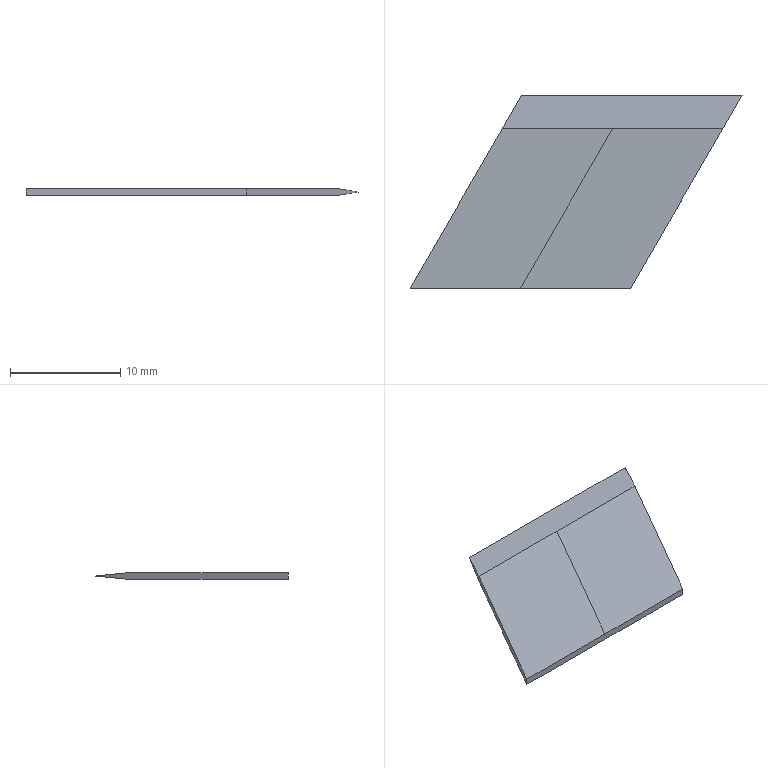Part | SolidWorks | features PLine 2, Extrusion 1, ICE 1, MirrorPattern 1 | 1 solid | 9 faces | box 30.104 x 17.5 x 0.6 mm | volume 192 mm3 | plane 9
STEP:
#1=CARTESIAN_POINT('',(10.,0.,0.6));
#2=VERTEX_POINT('',#1);
#3=CARTESIAN_POINT('',(18.372,14.5,0.6));
#4=VERTEX_POINT('',#3);
#5=CARTESIAN_POINT('',(7.5,-4.33,0.6));
#6=DIRECTION('',(0.5,0.866,0.));
#7=VECTOR('',#6,1000.);
#8=LINE('',#5,#7);
#9=EDGE_CURVE('',#2,#4,#8,.T.);
#10=ORIENTED_EDGE('',*,*,#9,.F.);
#11=CARTESIAN_POINT('',(20.,0.,0.6));
#12=VERTEX_POINT('',#11);
#13=CARTESIAN_POINT('',(20.,0.,0.6));
#14=DIRECTION('',(1.,0.,0.));
#15=VECTOR('',#14,1000.);
#16=LINE('',#13,#15);
#17=EDGE_CURVE('',#2,#12,#16,.T.);
#18=ORIENTED_EDGE('',*,*,#17,.T.);
#19=CARTESIAN_POINT('',(28.372,14.5,0.6));
#20=VERTEX_POINT('',#19);
#21=CARTESIAN_POINT('',(30.104,17.5,0.6));
#22=DIRECTION('',(0.5,0.866,0.));
#23=VECTOR('',#22,1000.);
#24=LINE('',#21,#23);
#25=EDGE_CURVE('',#12,#20,#24,.T.);
#26=ORIENTED_EDGE('',*,*,#25,.T.);
#27=CARTESIAN_POINT('',(30.104,14.5,0.6));
#28=DIRECTION('',(-1.,0.,0.));
#29=VECTOR('',#28,1000.);
#30=LINE('',#27,#29);
#31=EDGE_CURVE('',#20,#4,#30,.T.);
#32=ORIENTED_EDGE('',*,*,#31,.T.);
#33=EDGE_LOOP('',(#10,#18,#26,#32));
#34=FACE_OUTER_BOUND('',#33,.T.);
#35=CARTESIAN_POINT('',(0.,0.,0.6));
#36=DIRECTION('',(0.,0.,-1.));
#37=DIRECTION('',(-1.,0.,0.));
#38=AXIS2_PLACEMENT_3D('',#35,#36,#37);
#39=PLANE('',#38);
#40=ADVANCED_FACE('',(#34),#39,.F.);
#41=CARTESIAN_POINT('',(10.,0.,0.));
#42=VERTEX_POINT('',#41);
#43=CARTESIAN_POINT('',(20.,0.,0.));
#44=VERTEX_POINT('',#43);
#45=CARTESIAN_POINT('',(20.,0.,0.));
#46=DIRECTION('',(1.,0.,0.));
#47=VECTOR('',#46,1000.);
#48=LINE('',#45,#47);
#49=EDGE_CURVE('',#42,#44,#48,.T.);
#50=ORIENTED_EDGE('',*,*,#49,.F.);
#51=CARTESIAN_POINT('',(18.372,14.5,0.));
#52=VERTEX_POINT('',#51);
#53=CARTESIAN_POINT('',(7.5,-4.33,0.));
#54=DIRECTION('',(0.5,0.866,0.));
#55=VECTOR('',#54,1000.);
#56=LINE('',#53,#55);
#57=EDGE_CURVE('',#42,#52,#56,.T.);
#58=ORIENTED_EDGE('',*,*,#57,.T.);
#59=CARTESIAN_POINT('',(28.372,14.5,0.));
#60=VERTEX_POINT('',#59);
#61=CARTESIAN_POINT('',(0.,14.5,0.));
#62=DIRECTION('',(1.,0.,0.));
#63=VECTOR('',#62,1000.);
#64=LINE('',#61,#63);
#65=EDGE_CURVE('',#52,#60,#64,.T.);
#66=ORIENTED_EDGE('',*,*,#65,.T.);
#67=CARTESIAN_POINT('',(30.104,17.5,0.));
#68=DIRECTION('',(0.5,0.866,0.));
#69=VECTOR('',#68,1000.);
#70=LINE('',#67,#69);
#71=EDGE_CURVE('',#44,#60,#70,.T.);
#72=ORIENTED_EDGE('',*,*,#71,.F.);
#73=EDGE_LOOP('',(#50,#58,#66,#72));
#74=FACE_OUTER_BOUND('',#73,.T.);
#75=CARTESIAN_POINT('',(0.,0.,0.));
#76=DIRECTION('',(0.,0.,-1.));
#77=DIRECTION('',(-1.,0.,0.));
#78=AXIS2_PLACEMENT_3D('',#75,#76,#77);
#79=PLANE('',#78);
#80=ADVANCED_FACE('',(#74),#79,.T.);
#81=CARTESIAN_POINT('',(30.104,17.5,0.3));
#82=VERTEX_POINT('',#81);
#83=CARTESIAN_POINT('',(30.117,17.522,0.3022));
#84=DIRECTION('',(-0.4981,-0.8628,-0.08628));
#85=VECTOR('',#84,1000.);
#86=LINE('',#83,#85);
#87=EDGE_CURVE('',#82,#60,#86,.T.);
#88=ORIENTED_EDGE('',*,*,#87,.F.);
#89=CARTESIAN_POINT('',(30.091,17.478,0.3022));
#90=DIRECTION('',(-0.4981,-0.8628,0.08628));
#91=VECTOR('',#90,1000.);
#92=LINE('',#89,#91);
#93=EDGE_CURVE('',#82,#20,#92,.T.);
#94=ORIENTED_EDGE('',*,*,#93,.T.);
#95=ORIENTED_EDGE('',*,*,#25,.F.);
#96=CARTESIAN_POINT('',(20.,0.,0.6));
#97=DIRECTION('',(0.,0.,-1.));
#98=VECTOR('',#97,1000.);
#99=LINE('',#96,#98);
#100=EDGE_CURVE('',#12,#44,#99,.T.);
#101=ORIENTED_EDGE('',*,*,#100,.T.);
#102=ORIENTED_EDGE('',*,*,#71,.T.);
#103=EDGE_LOOP('',(#88,#94,#95,#101,#102));
#104=FACE_OUTER_BOUND('',#103,.T.);
#105=CARTESIAN_POINT('',(30.104,17.5,0.6));
#106=DIRECTION('',(-0.866,0.5,0.));
#107=DIRECTION('',(-0.5,-0.866,0.));
#108=AXIS2_PLACEMENT_3D('',#105,#106,#107);
#109=PLANE('',#108);
#110=ADVANCED_FACE('',(#104),#109,.F.);
#111=CARTESIAN_POINT('',(8.372,14.5,0.6));
#112=VERTEX_POINT('',#111);
#113=CARTESIAN_POINT('',(0.,0.,0.6));
#114=VERTEX_POINT('',#113);
#115=CARTESIAN_POINT('',(0.,0.,0.6));
#116=DIRECTION('',(-0.5,-0.866,0.));
#117=VECTOR('',#116,1000.);
#118=LINE('',#115,#117);
#119=EDGE_CURVE('',#112,#114,#118,.T.);
#120=ORIENTED_EDGE('',*,*,#119,.F.);
#121=CARTESIAN_POINT('',(10.104,17.5,0.3));
#122=VERTEX_POINT('',#121);
#123=CARTESIAN_POINT('',(0.06232,0.1079,2.039));
#124=DIRECTION('',(0.4981,0.8628,-0.08628));
#125=VECTOR('',#124,1000.);
#126=LINE('',#123,#125);
#127=EDGE_CURVE('',#112,#122,#126,.T.);
#128=ORIENTED_EDGE('',*,*,#127,.T.);
#129=CARTESIAN_POINT('',(8.372,14.5,0.));
#130=VERTEX_POINT('',#129);
#131=CARTESIAN_POINT('',(0.08811,0.1526,-1.435));
#132=DIRECTION('',(0.4981,0.8628,0.08628));
#133=VECTOR('',#132,1000.);
#134=LINE('',#131,#133);
#135=EDGE_CURVE('',#130,#122,#134,.T.);
#136=ORIENTED_EDGE('',*,*,#135,.F.);
#137=CARTESIAN_POINT('',(0.,0.,0.));
#138=VERTEX_POINT('',#137);
#139=CARTESIAN_POINT('',(0.,0.,0.));
#140=DIRECTION('',(-0.5,-0.866,0.));
#141=VECTOR('',#140,1000.);
#142=LINE('',#139,#141);
#143=EDGE_CURVE('',#130,#138,#142,.T.);
#144=ORIENTED_EDGE('',*,*,#143,.T.);
#145=CARTESIAN_POINT('',(0.,0.,0.6));
#146=DIRECTION('',(0.,0.,-1.));
#147=VECTOR('',#146,1000.);
#148=LINE('',#145,#147);
#149=EDGE_CURVE('',#114,#138,#148,.T.);
#150=ORIENTED_EDGE('',*,*,#149,.F.);
#151=EDGE_LOOP('',(#120,#128,#136,#144,#150));
#152=FACE_OUTER_BOUND('',#151,.T.);
#153=CARTESIAN_POINT('',(0.,0.,0.6));
#154=DIRECTION('',(0.866,-0.5,0.));
#155=DIRECTION('',(0.5,0.866,0.));
#156=AXIS2_PLACEMENT_3D('',#153,#154,#155);
#157=PLANE('',#156);
#158=ADVANCED_FACE('',(#152),#157,.F.);
#159=ORIENTED_EDGE('',*,*,#57,.F.);
#160=CARTESIAN_POINT('',(20.,0.,0.));
#161=DIRECTION('',(1.,0.,0.));
#162=VECTOR('',#161,1000.);
#163=LINE('',#160,#162);
#164=EDGE_CURVE('',#138,#42,#163,.T.);
#165=ORIENTED_EDGE('',*,*,#164,.F.);
#166=ORIENTED_EDGE('',*,*,#143,.F.);
#167=CARTESIAN_POINT('',(0.,14.5,0.));
#168=DIRECTION('',(1.,0.,0.));
#169=VECTOR('',#168,1000.);
#170=LINE('',#167,#169);
#171=EDGE_CURVE('',#130,#52,#170,.T.);
#172=ORIENTED_EDGE('',*,*,#171,.T.);
#173=EDGE_LOOP('',(#159,#165,#166,#172));
#174=FACE_OUTER_BOUND('',#173,.T.);
#175=CARTESIAN_POINT('',(0.,0.,0.));
#176=DIRECTION('',(0.,0.,-1.));
#177=DIRECTION('',(-1.,0.,0.));
#178=AXIS2_PLACEMENT_3D('',#175,#176,#177);
#179=PLANE('',#178);
#180=ADVANCED_FACE('',(#174),#179,.T.);
#181=ORIENTED_EDGE('',*,*,#164,.T.);
#182=ORIENTED_EDGE('',*,*,#49,.T.);
#183=ORIENTED_EDGE('',*,*,#100,.F.);
#184=ORIENTED_EDGE('',*,*,#17,.F.);
#185=CARTESIAN_POINT('',(20.,0.,0.6));
#186=DIRECTION('',(1.,0.,0.));
#187=VECTOR('',#186,1000.);
#188=LINE('',#185,#187);
#189=EDGE_CURVE('',#114,#2,#188,.T.);
#190=ORIENTED_EDGE('',*,*,#189,.F.);
#191=ORIENTED_EDGE('',*,*,#149,.T.);
#192=EDGE_LOOP('',(#181,#182,#183,#184,#190,#191));
#193=FACE_OUTER_BOUND('',#192,.T.);
#194=CARTESIAN_POINT('',(20.,0.,0.6));
#195=DIRECTION('',(0.,1.,0.));
#196=DIRECTION('',(-1.,0.,0.));
#197=AXIS2_PLACEMENT_3D('',#194,#195,#196);
#198=PLANE('',#197);
#199=ADVANCED_FACE('',(#193),#198,.F.);
#200=ORIENTED_EDGE('',*,*,#189,.T.);
#201=ORIENTED_EDGE('',*,*,#9,.T.);
#202=CARTESIAN_POINT('',(30.104,14.5,0.6));
#203=DIRECTION('',(-1.,0.,0.));
#204=VECTOR('',#203,1000.);
#205=LINE('',#202,#204);
#206=EDGE_CURVE('',#4,#112,#205,.T.);
#207=ORIENTED_EDGE('',*,*,#206,.T.);
#208=ORIENTED_EDGE('',*,*,#119,.T.);
#209=EDGE_LOOP('',(#200,#201,#207,#208));
#210=FACE_OUTER_BOUND('',#209,.T.);
#211=CARTESIAN_POINT('',(0.,0.,0.6));
#212=DIRECTION('',(0.,0.,-1.));
#213=DIRECTION('',(-1.,0.,0.));
#214=AXIS2_PLACEMENT_3D('',#211,#212,#213);
#215=PLANE('',#214);
#216=ADVANCED_FACE('',(#210),#215,.F.);
#217=ORIENTED_EDGE('',*,*,#87,.T.);
#218=ORIENTED_EDGE('',*,*,#65,.F.);
#219=ORIENTED_EDGE('',*,*,#171,.F.);
#220=ORIENTED_EDGE('',*,*,#135,.T.);
#221=CARTESIAN_POINT('',(30.104,17.5,0.3));
#222=DIRECTION('',(-1.,0.,0.));
#223=VECTOR('',#222,1000.);
#224=LINE('',#221,#223);
#225=EDGE_CURVE('',#82,#122,#224,.T.);
#226=ORIENTED_EDGE('',*,*,#225,.F.);
#227=EDGE_LOOP('',(#217,#218,#219,#220,#226));
#228=FACE_OUTER_BOUND('',#227,.T.);
#229=CARTESIAN_POINT('',(30.104,17.5,0.3));
#230=DIRECTION('',(0.,0.0995,-0.995));
#231=DIRECTION('',(0.,0.995,0.0995));
#232=AXIS2_PLACEMENT_3D('',#229,#230,#231);
#233=PLANE('',#232);
#234=ADVANCED_FACE('',(#228),#233,.T.);
#235=ORIENTED_EDGE('',*,*,#225,.T.);
#236=ORIENTED_EDGE('',*,*,#127,.F.);
#237=ORIENTED_EDGE('',*,*,#206,.F.);
#238=ORIENTED_EDGE('',*,*,#31,.F.);
#239=ORIENTED_EDGE('',*,*,#93,.F.);
#240=EDGE_LOOP('',(#235,#236,#237,#238,#239));
#241=FACE_OUTER_BOUND('',#240,.T.);
#242=CARTESIAN_POINT('',(30.104,17.5,0.3));
#243=DIRECTION('',(0.,-0.0995,-0.995));
#244=DIRECTION('',(0.,0.995,-0.0995));
#245=AXIS2_PLACEMENT_3D('',#242,#243,#244);
#246=PLANE('',#245);
#247=ADVANCED_FACE('',(#241),#246,.F.);
#248=CLOSED_SHELL('',(#40,#80,#110,#158,#180,#199,#216,#234,#247));
#249=MANIFOLD_SOLID_BREP('',#248);
#250=CARTESIAN_POINT('',(0.,0.,0.));
#251=DIRECTION('',(0.,0.,1.));
#252=DIRECTION('',(1.,0.,0.));
#253=AXIS2_PLACEMENT_3D('',#250,#251,#252);
#254=(LENGTH_UNIT()NAMED_UNIT(*)SI_UNIT(.MILLI.,.METRE.));
#255=UNCERTAINTY_MEASURE_WITH_UNIT(LENGTH_MEASURE(0.00001),#254,'','');
#256=(NAMED_UNIT(*)PLANE_ANGLE_UNIT()SI_UNIT($,.RADIAN.));
#257=(NAMED_UNIT(*)SI_UNIT($,.STERADIAN.)SOLID_ANGLE_UNIT());
#258=(GEOMETRIC_REPRESENTATION_CONTEXT(3)GLOBAL_UNCERTAINTY_ASSIGNED_CONTEXT((#255))GLOBAL_UNIT_ASSIGNED_CONTEXT((#254,#256,#257))REPRESENTATION_CONTEXT('',''));
#259=ADVANCED_BREP_SHAPE_REPRESENTATION('',(#249,#253),#258);